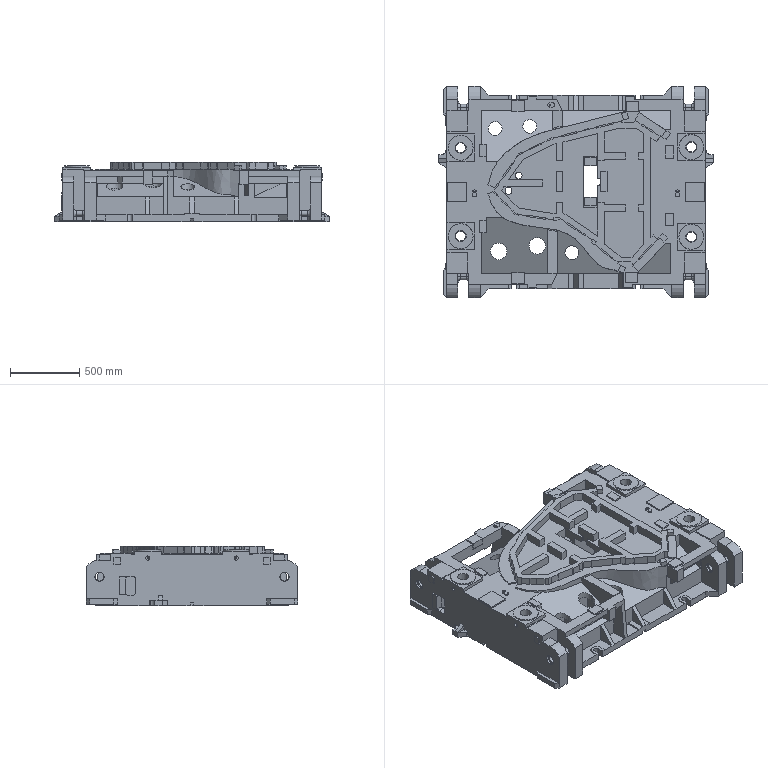Part | NX | features solid 2 | 1 solid | 1239 faces | box 1990 x 1530 x 430 mm | volume 378029427 mm3 | plane 1015 | cylinder 187 | spline 29 | torus 8 | commonest cylinder face diameters 68 x48 40 x44 30 x23 64 x16 60 x14 10 x10